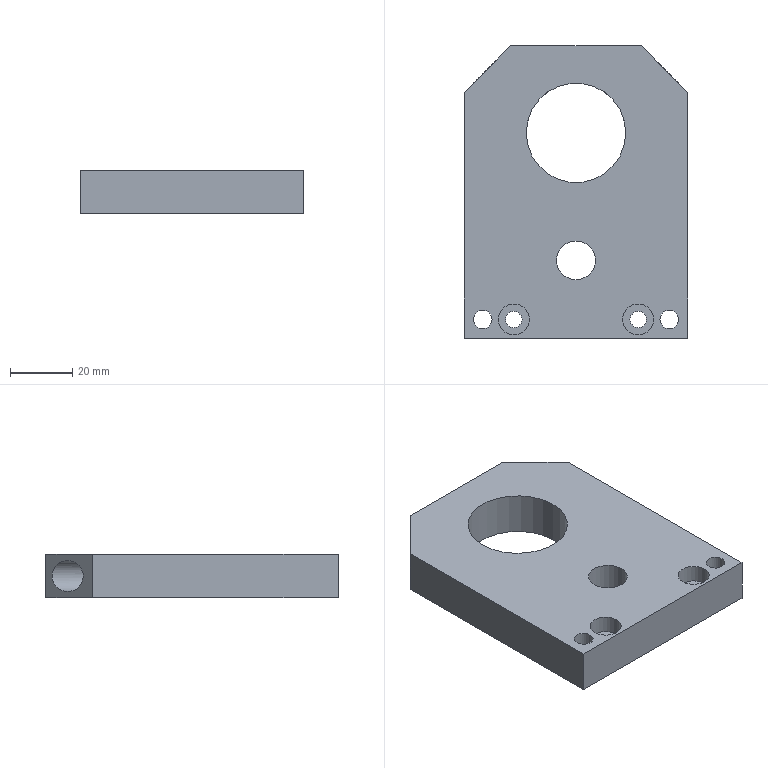Part | NX | 1 solid | 29 faces | box 72 x 94 x 14 mm | volume 74402 mm3 | plane 14 | cylinder 13 | cone 2 | commonest cylinder face diameters 10 x4 5.3 x2 5.5 x2 6 x2 4.2 x1 12.5 x1
STEP:
#1=CARTESIAN_POINT('',(22.65,-41.,0.));
#2=VERTEX_POINT('',#1);
#3=CARTESIAN_POINT('',(20.,-41.,0.));
#4=DIRECTION('',(0.,0.,-1.));
#5=DIRECTION('',(1.,0.,0.));
#6=AXIS2_PLACEMENT_3D('',#3,#4,#5);
#7=CIRCLE('',#6,2.65);
#8=EDGE_CURVE('',#2,#2,#7,.T.);
#9=ORIENTED_EDGE('',*,*,#8,.T.);
#10=EDGE_LOOP('',(#9));
#11=FACE_BOUND('',#10,.T.);
#12=CARTESIAN_POINT('',(22.65,-41.,8.3));
#13=VERTEX_POINT('',#12);
#14=CARTESIAN_POINT('',(20.,-41.,8.3));
#15=DIRECTION('',(0.,0.,1.));
#16=DIRECTION('',(1.,0.,0.));
#17=AXIS2_PLACEMENT_3D('',#14,#15,#16);
#18=CIRCLE('',#17,2.65);
#19=EDGE_CURVE('',#13,#13,#18,.T.);
#20=ORIENTED_EDGE('',*,*,#19,.T.);
#21=EDGE_LOOP('',(#20));
#22=FACE_BOUND('',#21,.T.);
#23=CARTESIAN_POINT('',(20.,-41.,0.));
#24=DIRECTION('',(0.,0.,1.));
#25=DIRECTION('',(-1.,0.,0.));
#26=AXIS2_PLACEMENT_3D('',#23,#24,#25);
#27=CYLINDRICAL_SURFACE('',#26,2.65);
#28=ADVANCED_FACE('',(#11,#22),#27,.F.);
#29=CARTESIAN_POINT('',(-6.25,-22.,14.));
#30=VERTEX_POINT('',#29);
#31=CARTESIAN_POINT('',(0.,-22.,14.));
#32=DIRECTION('',(0.,0.,-1.));
#33=DIRECTION('',(-1.,0.,0.));
#34=AXIS2_PLACEMENT_3D('',#31,#32,#33);
#35=CIRCLE('',#34,6.25);
#36=EDGE_CURVE('',#30,#30,#35,.T.);
#37=ORIENTED_EDGE('',*,*,#36,.T.);
#38=EDGE_LOOP('',(#37));
#39=FACE_BOUND('',#38,.T.);
#40=CARTESIAN_POINT('',(-27.,-41.,14.));
#41=VERTEX_POINT('',#40);
#42=CARTESIAN_POINT('',(-30.,-41.,14.));
#43=DIRECTION('',(0.,0.,1.));
#44=DIRECTION('',(1.,0.,0.));
#45=AXIS2_PLACEMENT_3D('',#42,#43,#44);
#46=CIRCLE('',#45,3.);
#47=EDGE_CURVE('',#41,#41,#46,.T.);
#48=ORIENTED_EDGE('',*,*,#47,.F.);
#49=EDGE_LOOP('',(#48));
#50=FACE_BOUND('',#49,.T.);
#51=CARTESIAN_POINT('',(16.,19.,14.));
#52=VERTEX_POINT('',#51);
#53=CARTESIAN_POINT('',(0.,19.,14.));
#54=DIRECTION('',(0.,0.,1.));
#55=DIRECTION('',(1.,0.,0.));
#56=AXIS2_PLACEMENT_3D('',#53,#54,#55);
#57=CIRCLE('',#56,16.);
#58=EDGE_CURVE('',#52,#52,#57,.T.);
#59=ORIENTED_EDGE('',*,*,#58,.F.);
#60=EDGE_LOOP('',(#59));
#61=FACE_BOUND('',#60,.T.);
#62=CARTESIAN_POINT('',(33.,-41.,14.));
#63=VERTEX_POINT('',#62);
#64=CARTESIAN_POINT('',(30.,-41.,14.));
#65=DIRECTION('',(0.,0.,1.));
#66=DIRECTION('',(1.,0.,0.));
#67=AXIS2_PLACEMENT_3D('',#64,#65,#66);
#68=CIRCLE('',#67,3.);
#69=EDGE_CURVE('',#63,#63,#68,.T.);
#70=ORIENTED_EDGE('',*,*,#69,.F.);
#71=EDGE_LOOP('',(#70));
#72=FACE_BOUND('',#71,.T.);
#73=CARTESIAN_POINT('',(-21.,47.,14.));
#74=VERTEX_POINT('',#73);
#75=CARTESIAN_POINT('',(-36.,32.,14.));
#76=VERTEX_POINT('',#75);
#77=CARTESIAN_POINT('',(-21.,47.,14.));
#78=DIRECTION('',(-0.7071,-0.7071,0.));
#79=VECTOR('',#78,1.);
#80=LINE('',#77,#79);
#81=EDGE_CURVE('',#74,#76,#80,.T.);
#82=ORIENTED_EDGE('',*,*,#81,.T.);
#83=CARTESIAN_POINT('',(-36.,-47.,14.));
#84=VERTEX_POINT('',#83);
#85=CARTESIAN_POINT('',(-36.,32.,14.));
#86=DIRECTION('',(0.,-1.,0.));
#87=VECTOR('',#86,1.);
#88=LINE('',#85,#87);
#89=EDGE_CURVE('',#76,#84,#88,.T.);
#90=ORIENTED_EDGE('',*,*,#89,.T.);
#91=CARTESIAN_POINT('',(36.,-47.,14.));
#92=VERTEX_POINT('',#91);
#93=CARTESIAN_POINT('',(-36.,-47.,14.));
#94=DIRECTION('',(1.,0.,0.));
#95=VECTOR('',#94,1.);
#96=LINE('',#93,#95);
#97=EDGE_CURVE('',#84,#92,#96,.T.);
#98=ORIENTED_EDGE('',*,*,#97,.T.);
#99=CARTESIAN_POINT('',(36.,32.,14.));
#100=VERTEX_POINT('',#99);
#101=CARTESIAN_POINT('',(36.,-47.,14.));
#102=DIRECTION('',(0.,1.,0.));
#103=VECTOR('',#102,1.);
#104=LINE('',#101,#103);
#105=EDGE_CURVE('',#92,#100,#104,.T.);
#106=ORIENTED_EDGE('',*,*,#105,.T.);
#107=CARTESIAN_POINT('',(21.,47.,14.));
#108=VERTEX_POINT('',#107);
#109=CARTESIAN_POINT('',(36.,32.,14.));
#110=DIRECTION('',(-0.7071,0.7071,0.));
#111=VECTOR('',#110,1.);
#112=LINE('',#109,#111);
#113=EDGE_CURVE('',#100,#108,#112,.T.);
#114=ORIENTED_EDGE('',*,*,#113,.T.);
#115=CARTESIAN_POINT('',(21.,47.,14.));
#116=DIRECTION('',(-1.,0.,0.));
#117=VECTOR('',#116,1.);
#118=LINE('',#115,#117);
#119=EDGE_CURVE('',#108,#74,#118,.T.);
#120=ORIENTED_EDGE('',*,*,#119,.T.);
#121=EDGE_LOOP('',(#82,#90,#98,#106,#114,#120));
#122=FACE_BOUND('',#121,.T.);
#123=CARTESIAN_POINT('',(-15.,-41.,14.));
#124=VERTEX_POINT('',#123);
#125=CARTESIAN_POINT('',(-20.,-41.,14.));
#126=DIRECTION('',(0.,0.,-1.));
#127=DIRECTION('',(1.,0.,0.));
#128=AXIS2_PLACEMENT_3D('',#125,#126,#127);
#129=CIRCLE('',#128,5.);
#130=EDGE_CURVE('',#124,#124,#129,.T.);
#131=ORIENTED_EDGE('',*,*,#130,.T.);
#132=EDGE_LOOP('',(#131));
#133=FACE_BOUND('',#132,.T.);
#134=CARTESIAN_POINT('',(25.,-41.,14.));
#135=VERTEX_POINT('',#134);
#136=CARTESIAN_POINT('',(20.,-41.,14.));
#137=DIRECTION('',(0.,0.,1.));
#138=DIRECTION('',(1.,0.,0.));
#139=AXIS2_PLACEMENT_3D('',#136,#137,#138);
#140=CIRCLE('',#139,5.);
#141=EDGE_CURVE('',#135,#135,#140,.T.);
#142=ORIENTED_EDGE('',*,*,#141,.F.);
#143=EDGE_LOOP('',(#142));
#144=FACE_BOUND('',#143,.T.);
#145=CARTESIAN_POINT('',(30.,-41.,14.));
#146=DIRECTION('',(0.,0.,1.));
#147=DIRECTION('',(-1.,0.,0.));
#148=AXIS2_PLACEMENT_3D('',#145,#146,#147);
#149=PLANE('',#148);
#150=ADVANCED_FACE('',(#39,#50,#61,#72,#122,#133,#144),#149,.T.);
#151=CARTESIAN_POINT('',(-33.,35.,7.));
#152=VERTEX_POINT('',#151);
#153=CARTESIAN_POINT('',(-28.,40.,7.));
#154=DIRECTION('',(0.7071,-0.7071,0.));
#155=DIRECTION('',(-0.7071,-0.7071,0.));
#156=AXIS2_PLACEMENT_3D('',#153,#154,#155);
#157=ELLIPSE('',#156,7.071,5.);
#158=EDGE_CURVE('',#152,#152,#157,.T.);
#159=ORIENTED_EDGE('',*,*,#158,.T.);
#160=EDGE_LOOP('',(#159));
#161=FACE_BOUND('',#160,.T.);
#162=ORIENTED_EDGE('',*,*,#81,.F.);
#163=CARTESIAN_POINT('',(-21.,47.,0.));
#164=VERTEX_POINT('',#163);
#165=CARTESIAN_POINT('',(-21.,47.,0.));
#166=DIRECTION('',(0.,0.,1.));
#167=VECTOR('',#166,1.);
#168=LINE('',#165,#167);
#169=EDGE_CURVE('',#164,#74,#168,.T.);
#170=ORIENTED_EDGE('',*,*,#169,.F.);
#171=CARTESIAN_POINT('',(-36.,32.,0.));
#172=VERTEX_POINT('',#171);
#173=CARTESIAN_POINT('',(-21.,47.,0.));
#174=DIRECTION('',(-0.7071,-0.7071,0.));
#175=VECTOR('',#174,1.);
#176=LINE('',#173,#175);
#177=EDGE_CURVE('',#164,#172,#176,.T.);
#178=ORIENTED_EDGE('',*,*,#177,.T.);
#179=CARTESIAN_POINT('',(-36.,32.,0.));
#180=DIRECTION('',(0.,0.,1.));
#181=VECTOR('',#180,1.);
#182=LINE('',#179,#181);
#183=EDGE_CURVE('',#172,#76,#182,.T.);
#184=ORIENTED_EDGE('',*,*,#183,.T.);
#185=EDGE_LOOP('',(#162,#170,#178,#184));
#186=FACE_BOUND('',#185,.T.);
#187=CARTESIAN_POINT('',(-21.,47.,0.));
#188=DIRECTION('',(-0.7071,0.7071,0.));
#189=DIRECTION('',(0.7071,0.7071,0.));
#190=AXIS2_PLACEMENT_3D('',#187,#188,#189);
#191=PLANE('',#190);
#192=ADVANCED_FACE('',(#161,#186),#191,.T.);
#193=ORIENTED_EDGE('',*,*,#89,.F.);
#194=ORIENTED_EDGE('',*,*,#183,.F.);
#195=CARTESIAN_POINT('',(-36.,-47.,0.));
#196=VERTEX_POINT('',#195);
#197=CARTESIAN_POINT('',(-36.,32.,0.));
#198=DIRECTION('',(0.,-1.,0.));
#199=VECTOR('',#198,1.);
#200=LINE('',#197,#199);
#201=EDGE_CURVE('',#172,#196,#200,.T.);
#202=ORIENTED_EDGE('',*,*,#201,.T.);
#203=CARTESIAN_POINT('',(-36.,-47.,0.));
#204=DIRECTION('',(0.,0.,1.));
#205=VECTOR('',#204,1.);
#206=LINE('',#203,#205);
#207=EDGE_CURVE('',#196,#84,#206,.T.);
#208=ORIENTED_EDGE('',*,*,#207,.T.);
#209=EDGE_LOOP('',(#193,#194,#202,#208));
#210=FACE_OUTER_BOUND('',#209,.T.);
#211=CARTESIAN_POINT('',(-36.,32.,0.));
#212=DIRECTION('',(-1.,0.,0.));
#213=DIRECTION('',(0.,0.,-1.));
#214=AXIS2_PLACEMENT_3D('',#211,#212,#213);
#215=PLANE('',#214);
#216=ADVANCED_FACE('',(#210),#215,.T.);
#217=ORIENTED_EDGE('',*,*,#97,.F.);
#218=ORIENTED_EDGE('',*,*,#207,.F.);
#219=CARTESIAN_POINT('',(36.,-47.,0.));
#220=VERTEX_POINT('',#219);
#221=CARTESIAN_POINT('',(-36.,-47.,0.));
#222=DIRECTION('',(1.,0.,0.));
#223=VECTOR('',#222,1.);
#224=LINE('',#221,#223);
#225=EDGE_CURVE('',#196,#220,#224,.T.);
#226=ORIENTED_EDGE('',*,*,#225,.T.);
#227=CARTESIAN_POINT('',(36.,-47.,0.));
#228=DIRECTION('',(0.,0.,1.));
#229=VECTOR('',#228,1.);
#230=LINE('',#227,#229);
#231=EDGE_CURVE('',#220,#92,#230,.T.);
#232=ORIENTED_EDGE('',*,*,#231,.T.);
#233=EDGE_LOOP('',(#217,#218,#226,#232));
#234=FACE_OUTER_BOUND('',#233,.T.);
#235=CARTESIAN_POINT('',(-36.,-47.,0.));
#236=DIRECTION('',(0.,-1.,0.));
#237=DIRECTION('',(0.,0.,1.));
#238=AXIS2_PLACEMENT_3D('',#235,#236,#237);
#239=PLANE('',#238);
#240=ADVANCED_FACE('',(#234),#239,.T.);
#241=ORIENTED_EDGE('',*,*,#105,.F.);
#242=ORIENTED_EDGE('',*,*,#231,.F.);
#243=CARTESIAN_POINT('',(36.,32.,0.));
#244=VERTEX_POINT('',#243);
#245=CARTESIAN_POINT('',(36.,-47.,0.));
#246=DIRECTION('',(0.,1.,0.));
#247=VECTOR('',#246,1.);
#248=LINE('',#245,#247);
#249=EDGE_CURVE('',#220,#244,#248,.T.);
#250=ORIENTED_EDGE('',*,*,#249,.T.);
#251=CARTESIAN_POINT('',(36.,32.,0.));
#252=DIRECTION('',(0.,0.,1.));
#253=VECTOR('',#252,1.);
#254=LINE('',#251,#253);
#255=EDGE_CURVE('',#244,#100,#254,.T.);
#256=ORIENTED_EDGE('',*,*,#255,.T.);
#257=EDGE_LOOP('',(#241,#242,#250,#256));
#258=FACE_OUTER_BOUND('',#257,.T.);
#259=CARTESIAN_POINT('',(36.,-47.,0.));
#260=DIRECTION('',(1.,0.,0.));
#261=DIRECTION('',(0.,0.,1.));
#262=AXIS2_PLACEMENT_3D('',#259,#260,#261);
#263=PLANE('',#262);
#264=ADVANCED_FACE('',(#258),#263,.T.);
#265=CARTESIAN_POINT('',(33.,35.,7.));
#266=VERTEX_POINT('',#265);
#267=CARTESIAN_POINT('',(28.,40.,7.));
#268=DIRECTION('',(-0.7071,-0.7071,0.));
#269=DIRECTION('',(0.7071,-0.7071,0.));
#270=AXIS2_PLACEMENT_3D('',#267,#268,#269);
#271=ELLIPSE('',#270,7.071,5.);
#272=EDGE_CURVE('',#266,#266,#271,.T.);
#273=ORIENTED_EDGE('',*,*,#272,.T.);
#274=EDGE_LOOP('',(#273));
#275=FACE_BOUND('',#274,.T.);
#276=ORIENTED_EDGE('',*,*,#113,.F.);
#277=ORIENTED_EDGE('',*,*,#255,.F.);
#278=CARTESIAN_POINT('',(21.,47.,0.));
#279=VERTEX_POINT('',#278);
#280=CARTESIAN_POINT('',(36.,32.,0.));
#281=DIRECTION('',(-0.7071,0.7071,0.));
#282=VECTOR('',#281,1.);
#283=LINE('',#280,#282);
#284=EDGE_CURVE('',#244,#279,#283,.T.);
#285=ORIENTED_EDGE('',*,*,#284,.T.);
#286=CARTESIAN_POINT('',(21.,47.,0.));
#287=DIRECTION('',(0.,0.,1.));
#288=VECTOR('',#287,1.);
#289=LINE('',#286,#288);
#290=EDGE_CURVE('',#279,#108,#289,.T.);
#291=ORIENTED_EDGE('',*,*,#290,.T.);
#292=EDGE_LOOP('',(#276,#277,#285,#291));
#293=FACE_BOUND('',#292,.T.);
#294=CARTESIAN_POINT('',(36.,32.,0.));
#295=DIRECTION('',(0.7071,0.7071,0.));
#296=DIRECTION('',(0.7071,-0.7071,0.));
#297=AXIS2_PLACEMENT_3D('',#294,#295,#296);
#298=PLANE('',#297);
#299=ADVANCED_FACE('',(#275,#293),#298,.T.);
#300=ORIENTED_EDGE('',*,*,#36,.F.);
#301=EDGE_LOOP('',(#300));
#302=FACE_BOUND('',#301,.T.);
#303=CARTESIAN_POINT('',(-6.25,-22.,0.));
#304=VERTEX_POINT('',#303);
#305=CARTESIAN_POINT('',(0.,-22.,0.));
#306=DIRECTION('',(0.,0.,-1.));
#307=DIRECTION('',(-1.,0.,0.));
#308=AXIS2_PLACEMENT_3D('',#305,#306,#307);
#309=CIRCLE('',#308,6.25);
#310=EDGE_CURVE('',#304,#304,#309,.T.);
#311=ORIENTED_EDGE('',*,*,#310,.T.);
#312=EDGE_LOOP('',(#311));
#313=FACE_BOUND('',#312,.T.);
#314=CARTESIAN_POINT('',(0.,-22.,0.));
#315=DIRECTION('',(0.,0.,1.));
#316=DIRECTION('',(-1.,0.,0.));
#317=AXIS2_PLACEMENT_3D('',#314,#315,#316);
#318=CYLINDRICAL_SURFACE('',#317,6.25);
#319=ADVANCED_FACE('',(#302,#313),#318,.F.);
#320=ORIENTED_EDGE('',*,*,#47,.T.);
#321=EDGE_LOOP('',(#320));
#322=FACE_BOUND('',#321,.T.);
#323=CARTESIAN_POINT('',(-27.,-41.,0.));
#324=VERTEX_POINT('',#323);
#325=CARTESIAN_POINT('',(-30.,-41.,0.));
#326=DIRECTION('',(0.,0.,1.));
#327=DIRECTION('',(1.,0.,0.));
#328=AXIS2_PLACEMENT_3D('',#325,#326,#327);
#329=CIRCLE('',#328,3.);
#330=EDGE_CURVE('',#324,#324,#329,.T.);
#331=ORIENTED_EDGE('',*,*,#330,.F.);
#332=EDGE_LOOP('',(#331));
#333=FACE_BOUND('',#332,.T.);
#334=CARTESIAN_POINT('',(-30.,-41.,0.));
#335=DIRECTION('',(0.,0.,1.));
#336=DIRECTION('',(-1.,0.,0.));
#337=AXIS2_PLACEMENT_3D('',#334,#335,#336);
#338=CYLINDRICAL_SURFACE('',#337,3.);
#339=ADVANCED_FACE('',(#322,#333),#338,.F.);
#340=CARTESIAN_POINT('',(-22.65,-41.,8.3));
#341=VERTEX_POINT('',#340);
#342=CARTESIAN_POINT('',(-20.,-41.,8.3));
#343=DIRECTION('',(0.,0.,1.));
#344=DIRECTION('',(-1.,0.,0.));
#345=AXIS2_PLACEMENT_3D('',#342,#343,#344);
#346=CIRCLE('',#345,2.65);
#347=EDGE_CURVE('',#341,#341,#346,.T.);
#348=ORIENTED_EDGE('',*,*,#347,.T.);
#349=EDGE_LOOP('',(#348));
#350=FACE_BOUND('',#349,.T.);
#351=CARTESIAN_POINT('',(-17.35,-41.,0.));
#352=VERTEX_POINT('',#351);
#353=CARTESIAN_POINT('',(-20.,-41.,0.));
#354=DIRECTION('',(0.,0.,1.));
#355=DIRECTION('',(1.,0.,0.));
#356=AXIS2_PLACEMENT_3D('',#353,#354,#355);
#357=CIRCLE('',#356,2.65);
#358=EDGE_CURVE('',#352,#352,#357,.T.);
#359=ORIENTED_EDGE('',*,*,#358,.F.);
#360=EDGE_LOOP('',(#359));
#361=FACE_BOUND('',#360,.T.);
#362=CARTESIAN_POINT('',(-20.,-41.,0.));
#363=DIRECTION('',(0.,0.,1.));
#364=DIRECTION('',(-1.,0.,0.));
#365=AXIS2_PLACEMENT_3D('',#362,#363,#364);
#366=CYLINDRICAL_SURFACE('',#365,2.65);
#367=ADVANCED_FACE('',(#350,#361),#366,.F.);
#368=ORIENTED_EDGE('',*,*,#58,.T.);
#369=EDGE_LOOP('',(#368));
#370=FACE_BOUND('',#369,.T.);
#371=CARTESIAN_POINT('',(16.,19.,0.));
#372=VERTEX_POINT('',#371);
#373=CARTESIAN_POINT('',(0.,19.,0.));
#374=DIRECTION('',(0.,0.,1.));
#375=DIRECTION('',(1.,0.,0.));
#376=AXIS2_PLACEMENT_3D('',#373,#374,#375);
#377=CIRCLE('',#376,16.);
#378=EDGE_CURVE('',#372,#372,#377,.T.);
#379=ORIENTED_EDGE('',*,*,#378,.F.);
#380=EDGE_LOOP('',(#379));
#381=FACE_BOUND('',#380,.T.);
#382=CARTESIAN_POINT('',(0.,19.,0.));
#383=DIRECTION('',(0.,0.,1.));
#384=DIRECTION('',(-1.,0.,0.));
#385=AXIS2_PLACEMENT_3D('',#382,#383,#384);
#386=CYLINDRICAL_SURFACE('',#385,16.);
#387=ADVANCED_FACE('',(#370,#381),#386,.F.);
#388=ORIENTED_EDGE('',*,*,#69,.T.);
#389=EDGE_LOOP('',(#388));
#390=FACE_BOUND('',#389,.T.);
#391=CARTESIAN_POINT('',(33.,-41.,0.));
#392=VERTEX_POINT('',#391);
#393=CARTESIAN_POINT('',(30.,-41.,0.));
#394=DIRECTION('',(0.,0.,1.));
#395=DIRECTION('',(1.,0.,0.));
#396=AXIS2_PLACEMENT_3D('',#393,#394,#395);
#397=CIRCLE('',#396,3.);
#398=EDGE_CURVE('',#392,#392,#397,.T.);
#399=ORIENTED_EDGE('',*,*,#398,.F.);
#400=EDGE_LOOP('',(#399));
#401=FACE_BOUND('',#400,.T.);
#402=CARTESIAN_POINT('',(30.,-41.,0.));
#403=DIRECTION('',(0.,0.,1.));
#404=DIRECTION('',(-1.,0.,0.));
#405=AXIS2_PLACEMENT_3D('',#402,#403,#404);
#406=CYLINDRICAL_SURFACE('',#405,3.);
#407=ADVANCED_FACE('',(#390,#401),#406,.F.);
#408=ORIENTED_EDGE('',*,*,#119,.F.);
#409=ORIENTED_EDGE('',*,*,#290,.F.);
#410=CARTESIAN_POINT('',(21.,47.,0.));
#411=DIRECTION('',(-1.,0.,0.));
#412=VECTOR('',#411,1.);
#413=LINE('',#410,#412);
#414=EDGE_CURVE('',#279,#164,#413,.T.);
#415=ORIENTED_EDGE('',*,*,#414,.T.);
#416=ORIENTED_EDGE('',*,*,#169,.T.);
#417=EDGE_LOOP('',(#408,#409,#415,#416));
#418=FACE_OUTER_BOUND('',#417,.T.);
#419=CARTESIAN_POINT('',(21.,47.,0.));
#420=DIRECTION('',(0.,1.,0.));
#421=DIRECTION('',(0.,0.,-1.));
#422=AXIS2_PLACEMENT_3D('',#419,#420,#421);
#423=PLANE('',#422);
#424=ADVANCED_FACE('',(#418),#423,.T.);
#425=ORIENTED_EDGE('',*,*,#177,.F.);
#426=ORIENTED_EDGE('',*,*,#414,.F.);
#427=ORIENTED_EDGE('',*,*,#284,.F.);
#428=ORIENTED_EDGE('',*,*,#249,.F.);
#429=ORIENTED_EDGE('',*,*,#225,.F.);
#430=ORIENTED_EDGE('',*,*,#201,.F.);
#431=EDGE_LOOP('',(#425,#426,#427,#428,#429,#430));
#432=FACE_BOUND('',#431,.T.);
#433=ORIENTED_EDGE('',*,*,#398,.T.);
#434=EDGE_LOOP('',(#433));
#435=FACE_BOUND('',#434,.T.);
#436=ORIENTED_EDGE('',*,*,#378,.T.);
#437=EDGE_LOOP('',(#436));
#438=FACE_BOUND('',#437,.T.);
#439=ORIENTED_EDGE('',*,*,#358,.T.);
#440=EDGE_LOOP('',(#439));
#441=FACE_BOUND('',#440,.T.);
#442=ORIENTED_EDGE('',*,*,#330,.T.);
#443=EDGE_LOOP('',(#442));
#444=FACE_BOUND('',#443,.T.);
#445=ORIENTED_EDGE('',*,*,#310,.F.);
#446=EDGE_LOOP('',(#445));
#447=FACE_BOUND('',#446,.T.);
#448=ORIENTED_EDGE('',*,*,#8,.F.);
#449=EDGE_LOOP('',(#448));
#450=FACE_BOUND('',#449,.T.);
#451=CARTESIAN_POINT('',(30.,-41.,0.));
#452=DIRECTION('',(0.,0.,1.));
#453=DIRECTION('',(-1.,0.,0.));
#454=AXIS2_PLACEMENT_3D('',#451,#452,#453);
#455=PLANE('',#454);
#456=ADVANCED_FACE('',(#432,#435,#438,#441,#444,#447,#450),#455,.F.);
#457=CARTESIAN_POINT('',(-15.,-41.,8.3));
#458=VERTEX_POINT('',#457);
#459=CARTESIAN_POINT('',(-20.,-41.,8.3));
#460=DIRECTION('',(0.,0.,1.));
#461=DIRECTION('',(1.,0.,0.));
#462=AXIS2_PLACEMENT_3D('',#459,#460,#461);
#463=CIRCLE('',#462,5.);
#464=EDGE_CURVE('',#458,#458,#463,.T.);
#465=ORIENTED_EDGE('',*,*,#464,.T.);
#466=EDGE_LOOP('',(#465));
#467=FACE_BOUND('',#466,.T.);
#468=ORIENTED_EDGE('',*,*,#347,.F.);
#469=EDGE_LOOP('',(#468));
#470=FACE_BOUND('',#469,.T.);
#471=CARTESIAN_POINT('',(-20.,-41.,8.3));
#472=DIRECTION('',(0.,0.,-1.));
#473=DIRECTION('',(1.,0.,0.));
#474=AXIS2_PLACEMENT_3D('',#471,#472,#473);
#475=PLANE('',#474);
#476=ADVANCED_FACE('',(#467,#470),#475,.F.);
#477=ORIENTED_EDGE('',*,*,#130,.F.);
#478=EDGE_LOOP('',(#477));
#479=FACE_BOUND('',#478,.T.);
#480=ORIENTED_EDGE('',*,*,#464,.F.);
#481=EDGE_LOOP('',(#480));
#482=FACE_BOUND('',#481,.T.);
#483=CARTESIAN_POINT('',(-20.,-41.,8.3));
#484=DIRECTION('',(0.,0.,1.));
#485=DIRECTION('',(-1.,0.,0.));
#486=AXIS2_PLACEMENT_3D('',#483,#484,#485);
#487=CYLINDRICAL_SURFACE('',#486,5.);
#488=ADVANCED_FACE('',(#479,#482),#487,.F.);
#489=ORIENTED_EDGE('',*,*,#141,.T.);
#490=EDGE_LOOP('',(#489));
#491=FACE_BOUND('',#490,.T.);
#492=CARTESIAN_POINT('',(25.,-41.,8.3));
#493=VERTEX_POINT('',#492);
#494=CARTESIAN_POINT('',(20.,-41.,8.3));
#495=DIRECTION('',(0.,0.,-1.));
#496=DIRECTION('',(1.,0.,0.));
#497=AXIS2_PLACEMENT_3D('',#494,#495,#496);
#498=CIRCLE('',#497,5.);
#499=EDGE_CURVE('',#493,#493,#498,.T.);
#500=ORIENTED_EDGE('',*,*,#499,.T.);
#501=EDGE_LOOP('',(#500));
#502=FACE_BOUND('',#501,.T.);
#503=CARTESIAN_POINT('',(20.,-41.,8.3));
#504=DIRECTION('',(0.,0.,1.));
#505=DIRECTION('',(-1.,0.,0.));
#506=AXIS2_PLACEMENT_3D('',#503,#504,#505);
#507=CYLINDRICAL_SURFACE('',#506,5.);
#508=ADVANCED_FACE('',(#491,#502),#507,.F.);
#509=ORIENTED_EDGE('',*,*,#19,.F.);
#510=EDGE_LOOP('',(#509));
#511=FACE_BOUND('',#510,.T.);
#512=ORIENTED_EDGE('',*,*,#499,.F.);
#513=EDGE_LOOP('',(#512));
#514=FACE_BOUND('',#513,.T.);
#515=CARTESIAN_POINT('',(20.,-41.,8.3));
#516=DIRECTION('',(0.,0.,1.));
#517=DIRECTION('',(-1.,0.,0.));
#518=AXIS2_PLACEMENT_3D('',#515,#516,#517);
#519=PLANE('',#518);
#520=ADVANCED_FACE('',(#511,#514),#519,.T.);
#521=ORIENTED_EDGE('',*,*,#272,.F.);
#522=EDGE_LOOP('',(#521));
#523=FACE_BOUND('',#522,.T.);
#524=CARTESIAN_POINT('',(28.,30.,12.));
#525=VERTEX_POINT('',#524);
#526=CARTESIAN_POINT('',(28.,30.,7.));
#527=DIRECTION('',(0.,-1.,0.));
#528=DIRECTION('',(0.,0.,1.));
#529=AXIS2_PLACEMENT_3D('',#526,#527,#528);
#530=CIRCLE('',#529,5.);
#531=EDGE_CURVE('',#525,#525,#530,.T.);
#532=ORIENTED_EDGE('',*,*,#531,.T.);
#533=EDGE_LOOP('',(#532));
#534=FACE_BOUND('',#533,.T.);
#535=CARTESIAN_POINT('',(28.,47.,7.));
#536=DIRECTION('',(0.,-1.,0.));
#537=DIRECTION('',(0.,0.,1.));
#538=AXIS2_PLACEMENT_3D('',#535,#536,#537);
#539=CYLINDRICAL_SURFACE('',#538,5.);
#540=ADVANCED_FACE('',(#523,#534),#539,.F.);
#541=CARTESIAN_POINT('',(28.,30.,9.75));
#542=VERTEX_POINT('',#541);
#543=CARTESIAN_POINT('',(28.,30.,7.));
#544=DIRECTION('',(0.,-1.,0.));
#545=DIRECTION('',(0.,0.,1.));
#546=AXIS2_PLACEMENT_3D('',#543,#544,#545);
#547=CIRCLE('',#546,2.75);
#548=EDGE_CURVE('',#542,#542,#547,.T.);
#549=ORIENTED_EDGE('',*,*,#548,.T.);
#550=EDGE_LOOP('',(#549));
#551=FACE_BOUND('',#550,.T.);
#552=ORIENTED_EDGE('',*,*,#531,.F.);
#553=EDGE_LOOP('',(#552));
#554=FACE_BOUND('',#553,.T.);
#555=CARTESIAN_POINT('',(28.,30.,7.));
#556=DIRECTION('',(0.,1.,0.));
#557=DIRECTION('',(0.,0.,-1.));
#558=AXIS2_PLACEMENT_3D('',#555,#556,#557);
#559=PLANE('',#558);
#560=ADVANCED_FACE('',(#551,#554),#559,.T.);
#561=ORIENTED_EDGE('',*,*,#158,.F.);
#562=EDGE_LOOP('',(#561));
#563=FACE_BOUND('',#562,.T.);
#564=CARTESIAN_POINT('',(-28.,30.,12.));
#565=VERTEX_POINT('',#564);
#566=CARTESIAN_POINT('',(-28.,30.,7.));
#567=DIRECTION('',(0.,-1.,0.));
#568=DIRECTION('',(0.,0.,1.));
#569=AXIS2_PLACEMENT_3D('',#566,#567,#568);
#570=CIRCLE('',#569,5.);
#571=EDGE_CURVE('',#565,#565,#570,.T.);
#572=ORIENTED_EDGE('',*,*,#571,.T.);
#573=EDGE_LOOP('',(#572));
#574=FACE_BOUND('',#573,.T.);
#575=CARTESIAN_POINT('',(-28.,47.,7.));
#576=DIRECTION('',(0.,-1.,0.));
#577=DIRECTION('',(0.,0.,1.));
#578=AXIS2_PLACEMENT_3D('',#575,#576,#577);
#579=CYLINDRICAL_SURFACE('',#578,5.);
#580=ADVANCED_FACE('',(#563,#574),#579,.F.);
#581=CARTESIAN_POINT('',(-28.,30.,9.75));
#582=VERTEX_POINT('',#581);
#583=CARTESIAN_POINT('',(-28.,30.,7.));
#584=DIRECTION('',(0.,-1.,0.));
#585=DIRECTION('',(0.,0.,1.));
#586=AXIS2_PLACEMENT_3D('',#583,#584,#585);
#587=CIRCLE('',#586,2.75);
#588=EDGE_CURVE('',#582,#582,#587,.T.);
#589=ORIENTED_EDGE('',*,*,#588,.T.);
#590=EDGE_LOOP('',(#589));
#591=FACE_BOUND('',#590,.T.);
#592=ORIENTED_EDGE('',*,*,#571,.F.);
#593=EDGE_LOOP('',(#592));
#594=FACE_BOUND('',#593,.T.);
#595=CARTESIAN_POINT('',(-28.,30.,7.));
#596=DIRECTION('',(0.,1.,0.));
#597=DIRECTION('',(0.,0.,-1.));
#598=AXIS2_PLACEMENT_3D('',#595,#596,#597);
#599=PLANE('',#598);
#600=ADVANCED_FACE('',(#591,#594),#599,.T.);
#601=CARTESIAN_POINT('',(-28.,19.,9.75));
#602=VERTEX_POINT('',#601);
#603=CARTESIAN_POINT('',(-28.,19.,7.));
#604=DIRECTION('',(0.,1.,0.));
#605=DIRECTION('',(0.,0.,1.));
#606=AXIS2_PLACEMENT_3D('',#603,#604,#605);
#607=CIRCLE('',#606,2.75);
#608=EDGE_CURVE('',#602,#602,#607,.T.);
#609=ORIENTED_EDGE('',*,*,#608,.F.);
#610=EDGE_LOOP('',(#609));
#611=FACE_BOUND('',#610,.T.);
#612=ORIENTED_EDGE('',*,*,#588,.F.);
#613=EDGE_LOOP('',(#612));
#614=FACE_BOUND('',#613,.T.);
#615=CARTESIAN_POINT('',(-28.,30.,7.));
#616=DIRECTION('',(0.,-1.,0.));
#617=DIRECTION('',(0.,0.,1.));
#618=AXIS2_PLACEMENT_3D('',#615,#616,#617);
#619=CYLINDRICAL_SURFACE('',#618,2.75);
#620=ADVANCED_FACE('',(#611,#614),#619,.F.);
#621=ORIENTED_EDGE('',*,*,#608,.T.);
#622=EDGE_LOOP('',(#621));
#623=FACE_OUTER_BOUND('',#622,.T.);
#624=CARTESIAN_POINT('',(-28.,19.,7.));
#625=DIRECTION('',(0.,-1.,0.));
#626=DIRECTION('',(0.,0.,1.));
#627=AXIS2_PLACEMENT_3D('',#624,#625,#626);
#628=PLANE('',#627);
#629=ADVANCED_FACE('',(#623),#628,.F.);
#630=CARTESIAN_POINT('',(28.,19.,9.75));
#631=VERTEX_POINT('',#630);
#632=CARTESIAN_POINT('',(28.,19.,7.));
#633=DIRECTION('',(0.,1.,0.));
#634=DIRECTION('',(0.,0.,1.));
#635=AXIS2_PLACEMENT_3D('',#632,#633,#634);
#636=CIRCLE('',#635,2.75);
#637=EDGE_CURVE('',#631,#631,#636,.T.);
#638=ORIENTED_EDGE('',*,*,#637,.F.);
#639=EDGE_LOOP('',(#638));
#640=FACE_BOUND('',#639,.T.);
#641=ORIENTED_EDGE('',*,*,#548,.F.);
#642=EDGE_LOOP('',(#641));
#643=FACE_BOUND('',#642,.T.);
#644=CARTESIAN_POINT('',(28.,30.,7.));
#645=DIRECTION('',(0.,-1.,0.));
#646=DIRECTION('',(0.,0.,1.));
#647=AXIS2_PLACEMENT_3D('',#644,#645,#646);
#648=CYLINDRICAL_SURFACE('',#647,2.75);
#649=ADVANCED_FACE('',(#640,#643),#648,.F.);
#650=CARTESIAN_POINT('',(28.,19.,4.5));
#651=VERTEX_POINT('',#650);
#652=CARTESIAN_POINT('',(28.,19.,7.));
#653=DIRECTION('',(0.,-1.,0.));
#654=DIRECTION('',(0.,0.,-1.));
#655=AXIS2_PLACEMENT_3D('',#652,#653,#654);
#656=CIRCLE('',#655,2.5);
#657=EDGE_CURVE('',#651,#651,#656,.T.);
#658=ORIENTED_EDGE('',*,*,#657,.T.);
#659=EDGE_LOOP('',(#658));
#660=FACE_BOUND('',#659,.T.);
#661=ORIENTED_EDGE('',*,*,#637,.T.);
#662=EDGE_LOOP('',(#661));
#663=FACE_BOUND('',#662,.T.);
#664=CARTESIAN_POINT('',(28.,19.,7.));
#665=DIRECTION('',(0.,-1.,0.));
#666=DIRECTION('',(0.,0.,1.));
#667=AXIS2_PLACEMENT_3D('',#664,#665,#666);
#668=PLANE('',#667);
#669=ADVANCED_FACE('',(#660,#663),#668,.F.);
#670=CARTESIAN_POINT('',(28.,18.6,4.9));
#671=VERTEX_POINT('',#670);
#672=CARTESIAN_POINT('',(28.,18.6,7.));
#673=DIRECTION('',(0.,1.,0.));
#674=DIRECTION('',(0.,0.,-1.));
#675=AXIS2_PLACEMENT_3D('',#672,#673,#674);
#676=CIRCLE('',#675,2.1);
#677=EDGE_CURVE('',#671,#671,#676,.T.);
#678=ORIENTED_EDGE('',*,*,#677,.T.);
#679=EDGE_LOOP('',(#678));
#680=FACE_BOUND('',#679,.T.);
#681=CARTESIAN_POINT('',(28.,14.,4.9));
#682=VERTEX_POINT('',#681);
#683=CARTESIAN_POINT('',(28.,14.,7.));
#684=DIRECTION('',(0.,1.,0.));
#685=DIRECTION('',(0.,0.,-1.));
#686=AXIS2_PLACEMENT_3D('',#683,#684,#685);
#687=CIRCLE('',#686,2.1);
#688=EDGE_CURVE('',#682,#682,#687,.T.);
#689=ORIENTED_EDGE('',*,*,#688,.F.);
#690=EDGE_LOOP('',(#689));
#691=FACE_BOUND('',#690,.T.);
#692=CARTESIAN_POINT('',(28.,30.,7.));
#693=DIRECTION('',(0.,-1.,0.));
#694=DIRECTION('',(0.,0.,1.));
#695=AXIS2_PLACEMENT_3D('',#692,#693,#694);
#696=CYLINDRICAL_SURFACE('',#695,2.1);
#697=ADVANCED_FACE('',(#680,#691),#696,.F.);
#698=ORIENTED_EDGE('',*,*,#688,.T.);
#699=EDGE_LOOP('',(#698));
#700=FACE_BOUND('',#699,.T.);
#701=CARTESIAN_POINT('',(28.,12.738,7.));
#702=VERTEX_POINT('',#701);
#703=VERTEX_LOOP('',#702);
#704=FACE_BOUND('',#703,.T.);
#705=CARTESIAN_POINT('',(28.,14.,7.));
#706=DIRECTION('',(0.,1.,0.));
#707=DIRECTION('',(0.,0.,-1.));
#708=AXIS2_PLACEMENT_3D('',#705,#706,#707);
#709=CONICAL_SURFACE('',#708,2.1,59.);
#710=ADVANCED_FACE('',(#700,#704),#709,.F.);
#711=ORIENTED_EDGE('',*,*,#677,.F.);
#712=EDGE_LOOP('',(#711));
#713=FACE_BOUND('',#712,.T.);
#714=ORIENTED_EDGE('',*,*,#657,.F.);
#715=EDGE_LOOP('',(#714));
#716=FACE_BOUND('',#715,.T.);
#717=CARTESIAN_POINT('',(28.,19.,7.));
#718=DIRECTION('',(0.,1.,0.));
#719=DIRECTION('',(0.,0.,-1.));
#720=AXIS2_PLACEMENT_3D('',#717,#718,#719);
#721=CONICAL_SURFACE('',#720,2.5,45.);
#722=ADVANCED_FACE('',(#713,#716),#721,.F.);
#723=CLOSED_SHELL('',(#28,#150,#192,#216,#240,#264,#299,#319,#339,#367,#387,#407,#424,#456,#476,#488,#508,#520,#540,#560,#580,#600,#620,#629,#649,#669,#697,#710,#722));
#724=MANIFOLD_SOLID_BREP('',#723);
#725=(LENGTH_UNIT()NAMED_UNIT(*)SI_UNIT(.MILLI.,.METRE.));
#726=UNCERTAINTY_MEASURE_WITH_UNIT(LENGTH_MEASURE(0.00002),#725,'','');
#727=(NAMED_UNIT(*)PLANE_ANGLE_UNIT()SI_UNIT($,.RADIAN.));
#728=PLANE_ANGLE_MEASURE_WITH_UNIT(PLANE_ANGLE_MEASURE(0.01745),#727);
#729=DIMENSIONAL_EXPONENTS(0.,0.,0.,0.,0.,0.,0.);
#730=(CONVERSION_BASED_UNIT('DEGREE',#728)NAMED_UNIT(#729)PLANE_ANGLE_UNIT());
#731=(NAMED_UNIT(*)SI_UNIT($,.STERADIAN.)SOLID_ANGLE_UNIT());
#732=(GEOMETRIC_REPRESENTATION_CONTEXT(3)GLOBAL_UNCERTAINTY_ASSIGNED_CONTEXT((#726))GLOBAL_UNIT_ASSIGNED_CONTEXT((#725,#730,#731))REPRESENTATION_CONTEXT('',''));
#733=ADVANCED_BREP_SHAPE_REPRESENTATION('',(#724),#732);